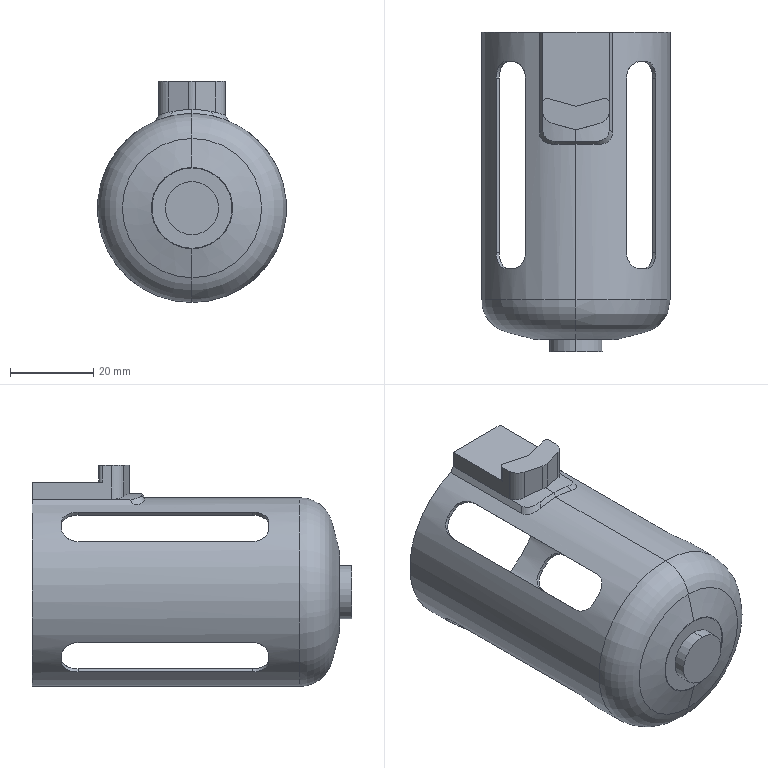Part | STEP file | AW30-03E_AW3020A Bowl_30 | 1 solid | 74 faces | box 45.5 x 76.9 x 53.25 mm | volume 11501 mm3 | cylinder 30 | plane 30 | cone 6 | torus 6 | spline 2 | commonest cylinder face diameters 8 x16 2 x3 6 x3 12.8 x2 43.5 x2 45.5 x2